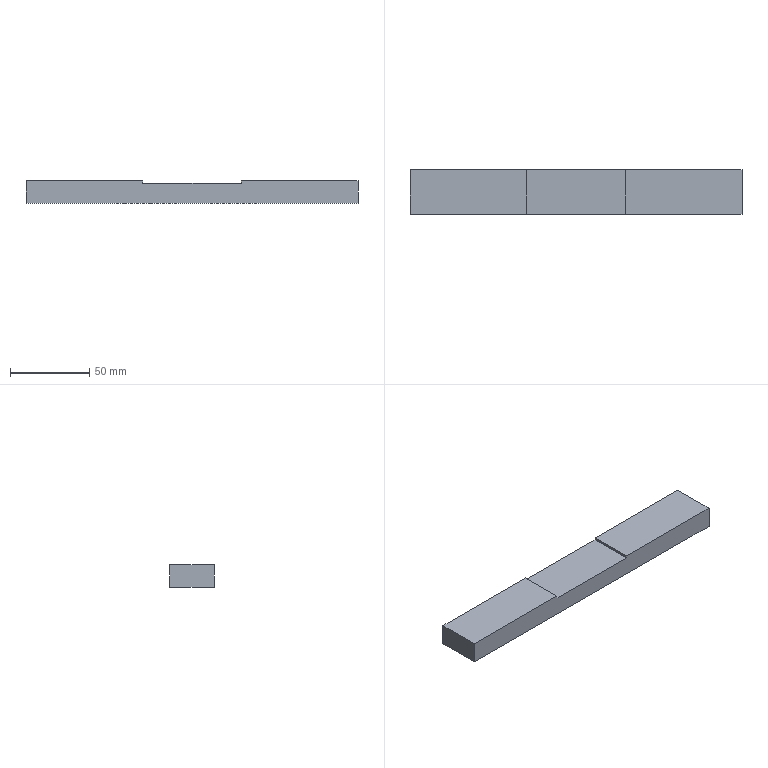Part | SolidWorks | features Extrusion 1, ICE 1 | 1 solid | 10 faces | box 210 x 28 x 14 mm | volume 79716 mm3 | plane 10
STEP:
#1=CARTESIAN_POINT('',(105.,14.,14.));
#2=VERTEX_POINT('',#1);
#3=CARTESIAN_POINT('',(31.,14.,14.));
#4=VERTEX_POINT('',#3);
#5=CARTESIAN_POINT('',(-105.,14.,14.));
#6=DIRECTION('',(-1.,0.,0.));
#7=VECTOR('',#6,1000.);
#8=LINE('',#5,#7);
#9=EDGE_CURVE('',#2,#4,#8,.T.);
#10=ORIENTED_EDGE('',*,*,#9,.T.);
#11=CARTESIAN_POINT('',(31.,-14.,14.));
#12=VERTEX_POINT('',#11);
#13=CARTESIAN_POINT('',(31.,-14.,14.));
#14=DIRECTION('',(0.,1.,0.));
#15=VECTOR('',#14,1000.);
#16=LINE('',#13,#15);
#17=EDGE_CURVE('',#12,#4,#16,.T.);
#18=ORIENTED_EDGE('',*,*,#17,.F.);
#19=CARTESIAN_POINT('',(105.,-14.,14.));
#20=VERTEX_POINT('',#19);
#21=CARTESIAN_POINT('',(-105.,-14.,14.));
#22=DIRECTION('',(1.,0.,0.));
#23=VECTOR('',#22,1000.);
#24=LINE('',#21,#23);
#25=EDGE_CURVE('',#12,#20,#24,.T.);
#26=ORIENTED_EDGE('',*,*,#25,.T.);
#27=CARTESIAN_POINT('',(105.,-14.,14.));
#28=DIRECTION('',(0.,1.,0.));
#29=VECTOR('',#28,1000.);
#30=LINE('',#27,#29);
#31=EDGE_CURVE('',#20,#2,#30,.T.);
#32=ORIENTED_EDGE('',*,*,#31,.T.);
#33=EDGE_LOOP('',(#10,#18,#26,#32));
#34=FACE_OUTER_BOUND('',#33,.T.);
#35=CARTESIAN_POINT('',(0.,0.,14.));
#36=DIRECTION('',(0.,0.,-1.));
#37=DIRECTION('',(-1.,0.,0.));
#38=AXIS2_PLACEMENT_3D('',#35,#36,#37);
#39=PLANE('',#38);
#40=ADVANCED_FACE('',(#34),#39,.F.);
#41=CARTESIAN_POINT('',(105.,-14.,0.));
#42=VERTEX_POINT('',#41);
#43=CARTESIAN_POINT('',(105.,14.,0.));
#44=VERTEX_POINT('',#43);
#45=CARTESIAN_POINT('',(105.,-14.,0.));
#46=DIRECTION('',(0.,1.,0.));
#47=VECTOR('',#46,1000.);
#48=LINE('',#45,#47);
#49=EDGE_CURVE('',#42,#44,#48,.T.);
#50=ORIENTED_EDGE('',*,*,#49,.T.);
#51=CARTESIAN_POINT('',(105.,14.,14.));
#52=DIRECTION('',(0.,0.,-1.));
#53=VECTOR('',#52,1000.);
#54=LINE('',#51,#53);
#55=EDGE_CURVE('',#2,#44,#54,.T.);
#56=ORIENTED_EDGE('',*,*,#55,.F.);
#57=ORIENTED_EDGE('',*,*,#31,.F.);
#58=CARTESIAN_POINT('',(105.,-14.,14.));
#59=DIRECTION('',(0.,0.,-1.));
#60=VECTOR('',#59,1000.);
#61=LINE('',#58,#60);
#62=EDGE_CURVE('',#20,#42,#61,.T.);
#63=ORIENTED_EDGE('',*,*,#62,.T.);
#64=EDGE_LOOP('',(#50,#56,#57,#63));
#65=FACE_OUTER_BOUND('',#64,.T.);
#66=CARTESIAN_POINT('',(105.,-14.,14.));
#67=DIRECTION('',(-1.,0.,0.));
#68=DIRECTION('',(0.,0.,1.));
#69=AXIS2_PLACEMENT_3D('',#66,#67,#68);
#70=PLANE('',#69);
#71=ADVANCED_FACE('',(#65),#70,.F.);
#72=CARTESIAN_POINT('',(31.,14.,12.5));
#73=VERTEX_POINT('',#72);
#74=CARTESIAN_POINT('',(-31.,14.,12.5));
#75=VERTEX_POINT('',#74);
#76=CARTESIAN_POINT('',(-31.,14.,12.5));
#77=DIRECTION('',(-1.,0.,0.));
#78=VECTOR('',#77,1000.);
#79=LINE('',#76,#78);
#80=EDGE_CURVE('',#73,#75,#79,.T.);
#81=ORIENTED_EDGE('',*,*,#80,.F.);
#82=CARTESIAN_POINT('',(31.,14.,12.5));
#83=DIRECTION('',(0.,0.,1.));
#84=VECTOR('',#83,1000.);
#85=LINE('',#82,#84);
#86=EDGE_CURVE('',#73,#4,#85,.T.);
#87=ORIENTED_EDGE('',*,*,#86,.T.);
#88=ORIENTED_EDGE('',*,*,#9,.F.);
#89=ORIENTED_EDGE('',*,*,#55,.T.);
#90=CARTESIAN_POINT('',(-105.,14.,0.));
#91=VERTEX_POINT('',#90);
#92=CARTESIAN_POINT('',(-105.,14.,0.));
#93=DIRECTION('',(-1.,0.,0.));
#94=VECTOR('',#93,1000.);
#95=LINE('',#92,#94);
#96=EDGE_CURVE('',#44,#91,#95,.T.);
#97=ORIENTED_EDGE('',*,*,#96,.T.);
#98=CARTESIAN_POINT('',(-105.,14.,14.));
#99=VERTEX_POINT('',#98);
#100=CARTESIAN_POINT('',(-105.,14.,14.));
#101=DIRECTION('',(0.,0.,-1.));
#102=VECTOR('',#101,1000.);
#103=LINE('',#100,#102);
#104=EDGE_CURVE('',#99,#91,#103,.T.);
#105=ORIENTED_EDGE('',*,*,#104,.F.);
#106=CARTESIAN_POINT('',(-31.,14.,14.));
#107=VERTEX_POINT('',#106);
#108=CARTESIAN_POINT('',(-105.,14.,14.));
#109=DIRECTION('',(-1.,0.,0.));
#110=VECTOR('',#109,1000.);
#111=LINE('',#108,#110);
#112=EDGE_CURVE('',#107,#99,#111,.T.);
#113=ORIENTED_EDGE('',*,*,#112,.F.);
#114=CARTESIAN_POINT('',(-31.,14.,12.5));
#115=DIRECTION('',(0.,0.,1.));
#116=VECTOR('',#115,1000.);
#117=LINE('',#114,#116);
#118=EDGE_CURVE('',#75,#107,#117,.T.);
#119=ORIENTED_EDGE('',*,*,#118,.F.);
#120=EDGE_LOOP('',(#81,#87,#88,#89,#97,#105,#113,#119));
#121=FACE_OUTER_BOUND('',#120,.T.);
#122=CARTESIAN_POINT('',(-105.,14.,14.));
#123=DIRECTION('',(0.,-1.,0.));
#124=DIRECTION('',(0.,0.,-1.));
#125=AXIS2_PLACEMENT_3D('',#122,#123,#124);
#126=PLANE('',#125);
#127=ADVANCED_FACE('',(#121),#126,.F.);
#128=CARTESIAN_POINT('',(-105.,-14.,0.));
#129=VERTEX_POINT('',#128);
#130=CARTESIAN_POINT('',(-105.,-14.,0.));
#131=DIRECTION('',(0.,-1.,0.));
#132=VECTOR('',#131,1000.);
#133=LINE('',#130,#132);
#134=EDGE_CURVE('',#91,#129,#133,.T.);
#135=ORIENTED_EDGE('',*,*,#134,.T.);
#136=CARTESIAN_POINT('',(-105.,-14.,14.));
#137=VERTEX_POINT('',#136);
#138=CARTESIAN_POINT('',(-105.,-14.,14.));
#139=DIRECTION('',(0.,0.,-1.));
#140=VECTOR('',#139,1000.);
#141=LINE('',#138,#140);
#142=EDGE_CURVE('',#137,#129,#141,.T.);
#143=ORIENTED_EDGE('',*,*,#142,.F.);
#144=CARTESIAN_POINT('',(-105.,-14.,14.));
#145=DIRECTION('',(0.,-1.,0.));
#146=VECTOR('',#145,1000.);
#147=LINE('',#144,#146);
#148=EDGE_CURVE('',#99,#137,#147,.T.);
#149=ORIENTED_EDGE('',*,*,#148,.F.);
#150=ORIENTED_EDGE('',*,*,#104,.T.);
#151=EDGE_LOOP('',(#135,#143,#149,#150));
#152=FACE_OUTER_BOUND('',#151,.T.);
#153=CARTESIAN_POINT('',(-105.,-14.,14.));
#154=DIRECTION('',(1.,0.,0.));
#155=DIRECTION('',(0.,0.,-1.));
#156=AXIS2_PLACEMENT_3D('',#153,#154,#155);
#157=PLANE('',#156);
#158=ADVANCED_FACE('',(#152),#157,.F.);
#159=ORIENTED_EDGE('',*,*,#25,.F.);
#160=CARTESIAN_POINT('',(31.,-14.,12.5));
#161=VERTEX_POINT('',#160);
#162=CARTESIAN_POINT('',(31.,-14.,12.5));
#163=DIRECTION('',(0.,0.,1.));
#164=VECTOR('',#163,1000.);
#165=LINE('',#162,#164);
#166=EDGE_CURVE('',#161,#12,#165,.T.);
#167=ORIENTED_EDGE('',*,*,#166,.F.);
#168=CARTESIAN_POINT('',(-31.,-14.,12.5));
#169=VERTEX_POINT('',#168);
#170=CARTESIAN_POINT('',(-31.,-14.,12.5));
#171=DIRECTION('',(1.,0.,0.));
#172=VECTOR('',#171,1000.);
#173=LINE('',#170,#172);
#174=EDGE_CURVE('',#169,#161,#173,.T.);
#175=ORIENTED_EDGE('',*,*,#174,.F.);
#176=CARTESIAN_POINT('',(-31.,-14.,14.));
#177=VERTEX_POINT('',#176);
#178=CARTESIAN_POINT('',(-31.,-14.,12.5));
#179=DIRECTION('',(0.,0.,1.));
#180=VECTOR('',#179,1000.);
#181=LINE('',#178,#180);
#182=EDGE_CURVE('',#169,#177,#181,.T.);
#183=ORIENTED_EDGE('',*,*,#182,.T.);
#184=CARTESIAN_POINT('',(-105.,-14.,14.));
#185=DIRECTION('',(1.,0.,0.));
#186=VECTOR('',#185,1000.);
#187=LINE('',#184,#186);
#188=EDGE_CURVE('',#137,#177,#187,.T.);
#189=ORIENTED_EDGE('',*,*,#188,.F.);
#190=ORIENTED_EDGE('',*,*,#142,.T.);
#191=CARTESIAN_POINT('',(-105.,-14.,0.));
#192=DIRECTION('',(1.,0.,0.));
#193=VECTOR('',#192,1000.);
#194=LINE('',#191,#193);
#195=EDGE_CURVE('',#129,#42,#194,.T.);
#196=ORIENTED_EDGE('',*,*,#195,.T.);
#197=ORIENTED_EDGE('',*,*,#62,.F.);
#198=EDGE_LOOP('',(#159,#167,#175,#183,#189,#190,#196,#197));
#199=FACE_OUTER_BOUND('',#198,.T.);
#200=CARTESIAN_POINT('',(-105.,-14.,14.));
#201=DIRECTION('',(0.,1.,0.));
#202=DIRECTION('',(0.,0.,1.));
#203=AXIS2_PLACEMENT_3D('',#200,#201,#202);
#204=PLANE('',#203);
#205=ADVANCED_FACE('',(#199),#204,.F.);
#206=ORIENTED_EDGE('',*,*,#188,.T.);
#207=CARTESIAN_POINT('',(-31.,-14.,14.));
#208=DIRECTION('',(0.,-1.,0.));
#209=VECTOR('',#208,1000.);
#210=LINE('',#207,#209);
#211=EDGE_CURVE('',#107,#177,#210,.T.);
#212=ORIENTED_EDGE('',*,*,#211,.F.);
#213=ORIENTED_EDGE('',*,*,#112,.T.);
#214=ORIENTED_EDGE('',*,*,#148,.T.);
#215=EDGE_LOOP('',(#206,#212,#213,#214));
#216=FACE_OUTER_BOUND('',#215,.T.);
#217=CARTESIAN_POINT('',(0.,0.,14.));
#218=DIRECTION('',(0.,0.,-1.));
#219=DIRECTION('',(-1.,0.,0.));
#220=AXIS2_PLACEMENT_3D('',#217,#218,#219);
#221=PLANE('',#220);
#222=ADVANCED_FACE('',(#216),#221,.F.);
#223=ORIENTED_EDGE('',*,*,#49,.F.);
#224=ORIENTED_EDGE('',*,*,#195,.F.);
#225=ORIENTED_EDGE('',*,*,#134,.F.);
#226=ORIENTED_EDGE('',*,*,#96,.F.);
#227=EDGE_LOOP('',(#223,#224,#225,#226));
#228=FACE_OUTER_BOUND('',#227,.T.);
#229=CARTESIAN_POINT('',(0.,0.,0.));
#230=DIRECTION('',(0.,0.,-1.));
#231=DIRECTION('',(-1.,0.,0.));
#232=AXIS2_PLACEMENT_3D('',#229,#230,#231);
#233=PLANE('',#232);
#234=ADVANCED_FACE('',(#228),#233,.T.);
#235=ORIENTED_EDGE('',*,*,#17,.T.);
#236=ORIENTED_EDGE('',*,*,#86,.F.);
#237=CARTESIAN_POINT('',(31.,-14.,12.5));
#238=DIRECTION('',(0.,1.,0.));
#239=VECTOR('',#238,1000.);
#240=LINE('',#237,#239);
#241=EDGE_CURVE('',#161,#73,#240,.T.);
#242=ORIENTED_EDGE('',*,*,#241,.F.);
#243=ORIENTED_EDGE('',*,*,#166,.T.);
#244=EDGE_LOOP('',(#235,#236,#242,#243));
#245=FACE_OUTER_BOUND('',#244,.T.);
#246=CARTESIAN_POINT('',(31.,-14.,12.5));
#247=DIRECTION('',(1.,0.,0.));
#248=DIRECTION('',(0.,0.,-1.));
#249=AXIS2_PLACEMENT_3D('',#246,#247,#248);
#250=PLANE('',#249);
#251=ADVANCED_FACE('',(#245),#250,.F.);
#252=ORIENTED_EDGE('',*,*,#211,.T.);
#253=ORIENTED_EDGE('',*,*,#182,.F.);
#254=CARTESIAN_POINT('',(-31.,-14.,12.5));
#255=DIRECTION('',(0.,-1.,0.));
#256=VECTOR('',#255,1000.);
#257=LINE('',#254,#256);
#258=EDGE_CURVE('',#75,#169,#257,.T.);
#259=ORIENTED_EDGE('',*,*,#258,.F.);
#260=ORIENTED_EDGE('',*,*,#118,.T.);
#261=EDGE_LOOP('',(#252,#253,#259,#260));
#262=FACE_OUTER_BOUND('',#261,.T.);
#263=CARTESIAN_POINT('',(-31.,-14.,12.5));
#264=DIRECTION('',(-1.,0.,0.));
#265=DIRECTION('',(0.,0.,1.));
#266=AXIS2_PLACEMENT_3D('',#263,#264,#265);
#267=PLANE('',#266);
#268=ADVANCED_FACE('',(#262),#267,.F.);
#269=ORIENTED_EDGE('',*,*,#241,.T.);
#270=ORIENTED_EDGE('',*,*,#80,.T.);
#271=ORIENTED_EDGE('',*,*,#258,.T.);
#272=ORIENTED_EDGE('',*,*,#174,.T.);
#273=EDGE_LOOP('',(#269,#270,#271,#272));
#274=FACE_OUTER_BOUND('',#273,.T.);
#275=CARTESIAN_POINT('',(0.,0.,12.5));
#276=DIRECTION('',(0.,0.,-1.));
#277=DIRECTION('',(-1.,0.,0.));
#278=AXIS2_PLACEMENT_3D('',#275,#276,#277);
#279=PLANE('',#278);
#280=ADVANCED_FACE('',(#274),#279,.F.);
#281=CLOSED_SHELL('',(#40,#71,#127,#158,#205,#222,#234,#251,#268,#280));
#282=MANIFOLD_SOLID_BREP('',#281);
#283=CARTESIAN_POINT('',(0.,0.,0.));
#284=DIRECTION('',(0.,0.,1.));
#285=DIRECTION('',(1.,0.,0.));
#286=AXIS2_PLACEMENT_3D('',#283,#284,#285);
#287=(LENGTH_UNIT()NAMED_UNIT(*)SI_UNIT(.MILLI.,.METRE.));
#288=UNCERTAINTY_MEASURE_WITH_UNIT(LENGTH_MEASURE(0.00001),#287,'','');
#289=(NAMED_UNIT(*)PLANE_ANGLE_UNIT()SI_UNIT($,.RADIAN.));
#290=(NAMED_UNIT(*)SI_UNIT($,.STERADIAN.)SOLID_ANGLE_UNIT());
#291=(GEOMETRIC_REPRESENTATION_CONTEXT(3)GLOBAL_UNCERTAINTY_ASSIGNED_CONTEXT((#288))GLOBAL_UNIT_ASSIGNED_CONTEXT((#287,#289,#290))REPRESENTATION_CONTEXT('',''));
#292=ADVANCED_BREP_SHAPE_REPRESENTATION('',(#282,#286),#291);